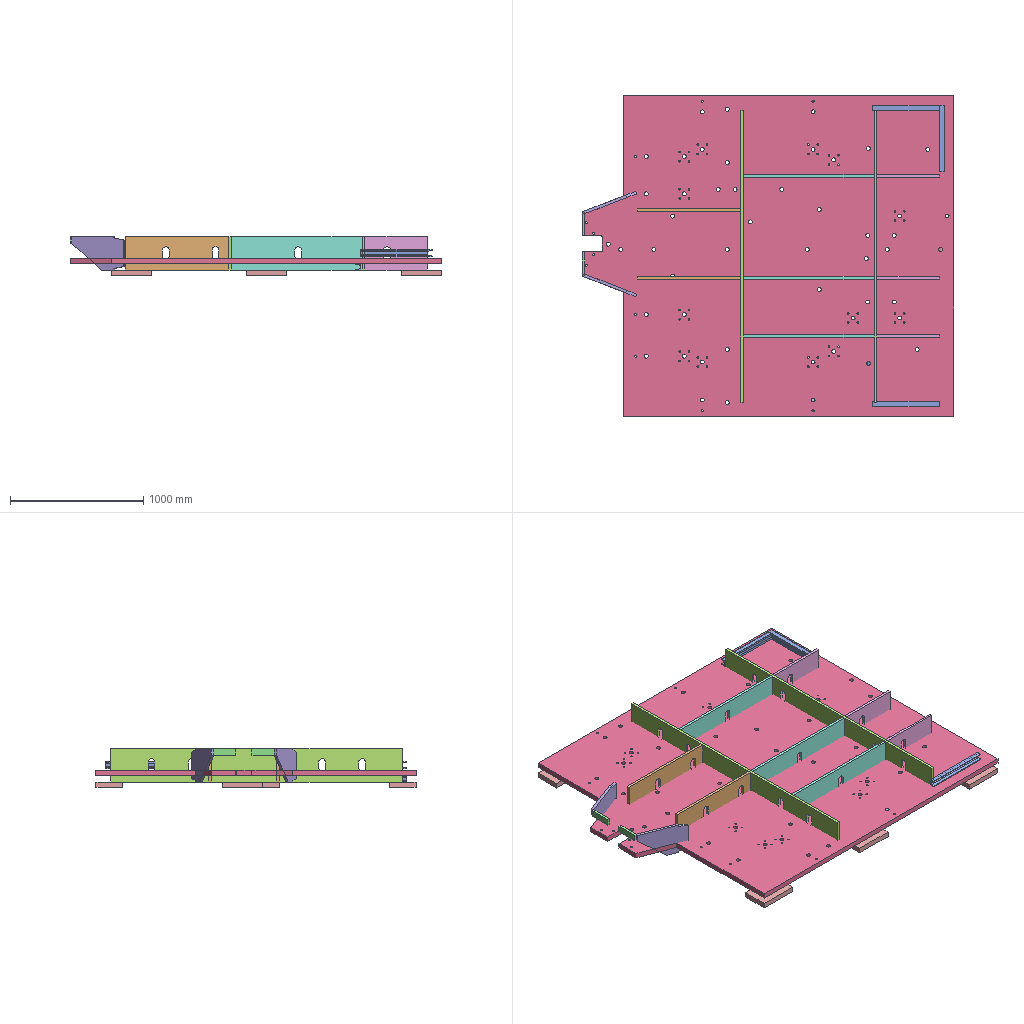Assembly | SolidWorks | 9 different items | 24 placed | box 2789 x 2400 x 290 mm
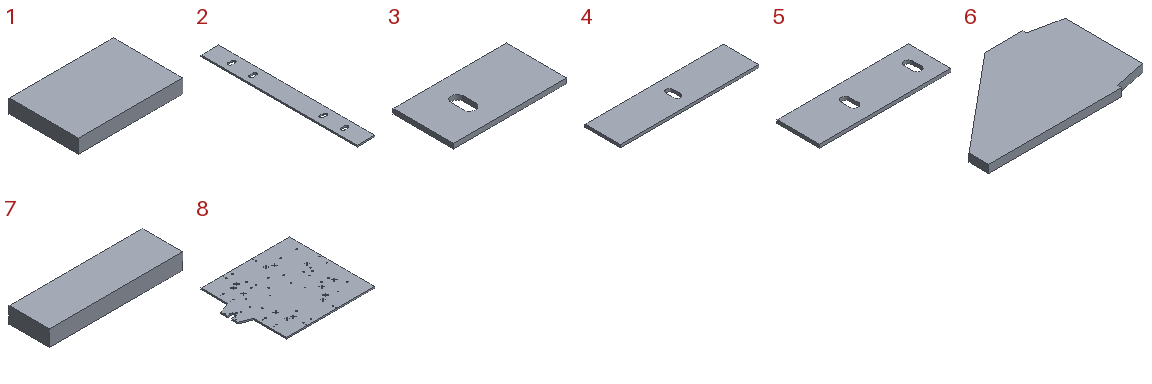Parts list (item | name | quantity | size | volume | features):
1 | - | x8 | 300 x 200 x 40 mm | 2400000 mm3 | features Extrusion 1
2 | - | x2 | 250 x 2186 x 20 mm | 10572920 mm3 | features Extrusion 1
3 | - | x3 | 468.5 x 250 x 20 mm | 2253231 mm3 | features Extrusion 1
4 | - | x3 | 980 x 250 x 20 mm | 4810730 mm3 | features Extrusion 1
5 | - | x2 | 775.098 x 250 x 20 mm | 3696953 mm3 | features Extrusion 1
6 | - | x2 | 416.402 x 250 x 20 mm | 1542694 mm3 | features Extrusion 1
7 | - | x2 | 166 x 50 x 20 mm | 166000 mm3 | features Extrusion 1
8 | - | x1 | 2789 x 2400 x 40 mm | 242886322 mm3 | features Extrusion 1
9 | hot-rolled steel channel gb | x1 | - | - | -
Mates (type | each side: item.copy, entity, surface, feature):
Coincident | assembly face | 1.1 face plane Boss-Extrude1 | 2 times
Coincident | 1.1 face plane Boss-Extrude1 | 1.2 face plane Boss-Extrude1
Coincident | 1.2 face plane Boss-Extrude1 | 1.3 face plane Boss-Extrude1
Coincident | 1.3 face plane Boss-Extrude1 | 1.4 face plane Boss-Extrude1
Coincident | 1.1 face plane Boss-Extrude1 | 1.5 face plane Boss-Extrude1
Coincident | 1.5 face plane Boss-Extrude1 | 1.6 face plane Boss-Extrude1 | 2 times
Coincident | 1.5 face plane Boss-Extrude1 | 1.7 face plane Boss-Extrude1
Coincident | 1.4 face plane Boss-Extrude1 | 1.8 face plane Boss-Extrude1
Coincident | assembly face | 1.3 face plane Boss-Extrude1 | 2 times
Coincident | assembly face | 1.8 face plane Boss-Extrude1 | 2 times
Coincident | assembly face | 1.6 face plane Boss-Extrude1 | 2 times
Coincident | assembly face | 2.1 face plane Boss-Extrude1
Coincident | assembly face | 2.2 face plane Boss-Extrude1
Coincident | assembly face | 3.1 face plane Boss-Extrude1
Coincident | assembly face | 3.2 face plane Boss-Extrude1
Coincident | assembly face | 3.3 face plane Boss-Extrude1
Coincident | 2.1 face plane Boss-Extrude1 | 3.1 face plane Boss-Extrude1
Coincident | assembly face | 4.1 face plane Boss-Extrude1
Coincident | assembly face | 4.2 face plane Boss-Extrude1
Coincident | assembly face | 4.3 face plane Boss-Extrude1
Coincident | 2.1 face plane Boss-Extrude1 | 4.1 face plane Boss-Extrude1
Coincident | 2.1 face plane Boss-Extrude1 | 4.2 face plane Boss-Extrude1
Coincident | 3.3 face plane Boss-Extrude1 | 4.2 face plane Boss-Extrude1
Coincident | 3.2 face plane Boss-Extrude1 | 4.1 face plane Boss-Extrude1
Coincident | 3.1 face plane Boss-Extrude1 | 4.3 face plane Boss-Extrude1
Coincident | 2.1 face plane Boss-Extrude1 | 4.3 face plane Boss-Extrude1
Coincident | assembly face | 5.1 face plane Boss-Extrude1
Coincident | assembly face | 5.2 face plane Boss-Extrude1
Coincident | 2.2 face plane Boss-Extrude1 | 4.2 face plane Boss-Extrude1
Coincident | 2.2 face plane Boss-Extrude1 | 5.2 face plane Boss-Extrude1
Coincident | 2.2 face plane Boss-Extrude1 | 5.1 face plane Boss-Extrude1
Coincident | 4.1 face plane Boss-Extrude1 | 5.1 face plane Boss-Extrude1
Coincident | assembly face | 7.1 face plane Boss-Extrude1 | 3 times
Coincident | assembly face | 7.2 face plane Boss-Extrude1 | 3 times
Coincident | assembly face | 6.1 face plane Boss-Extrude1
Coincident | assembly face | 6.2 face plane Boss-Extrude1
Coincident | assembly edge | 6.2 edge
Coincident | assembly edge | 6.1 edge
Coincident | 6.1 face plane Boss-Extrude1 | 7.2 edge
Coincident | 6.2 face plane Boss-Extrude1 | 7.1 edge
Coincident | assembly face | 1.4 face plane Boss-Extrude1
DistanceDim | 5.1 face plane Boss-Extrude1 | 5.2 face plane Boss-Extrude1
DistanceDim | 4.2 face plane Boss-Extrude1 | 4.1 face plane Boss-Extrude1
DistanceDim | 4.3 face plane Boss-Extrude1 | 5.2 face plane Boss-Extrude1
Coincident | assembly face | 1.2 face plane Boss-Extrude1
Coincident | assembly face | 1.7 face plane Boss-Extrude1
Coincident | 1.2 face plane Boss-Extrude1 | 1.7 face plane Boss-Extrude1
Coincident | 1.4 face plane Boss-Extrude1 | 3.2 face plane Boss-Extrude1
Coincident | 1.1 face plane Boss-Extrude1 | 8.1 face plane Boss-Extrude1 | 2 times